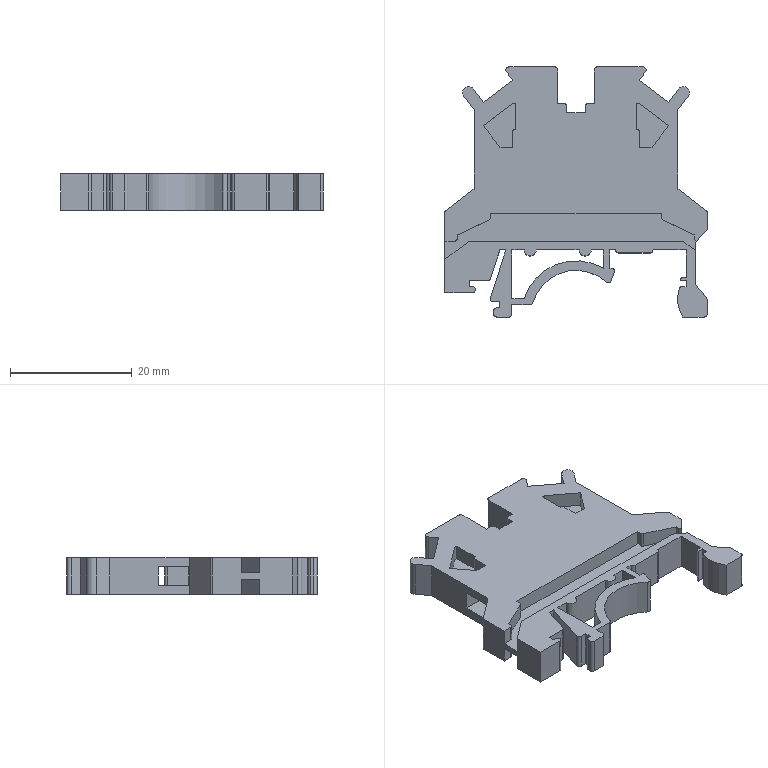Part | STEP file | terminal block UK2.5B | 1 solid | 213 faces | box 43 x 41 x 6 mm | volume 4189 mm3 | plane 152 | cylinder 61 | commonest cylinder face diameters 1 x49 2 x5 4 x4 11 x1 14.7 x1 17.837 x1